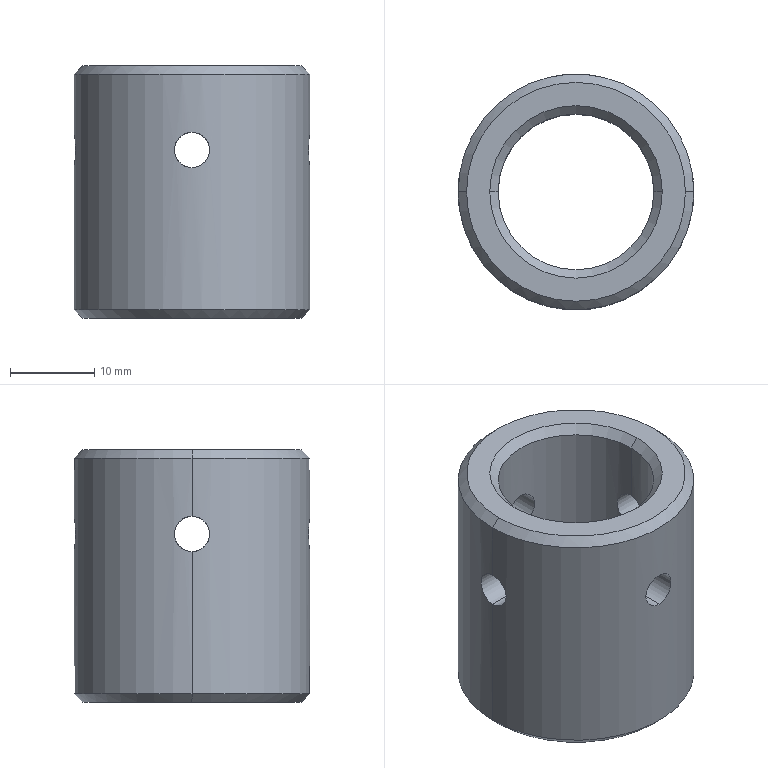Part | SolidWorks | features HoleWzd 5, Chamfer 1, Extrusion 1 | 1 solid | 38 faces | box 28 x 28 x 30 mm | volume 9846 mm3 | cylinder 20 | cone 16 | plane 2 | commonest cylinder face diameters 2.5 x8 4.2 x8 18.5 x2 28 x2